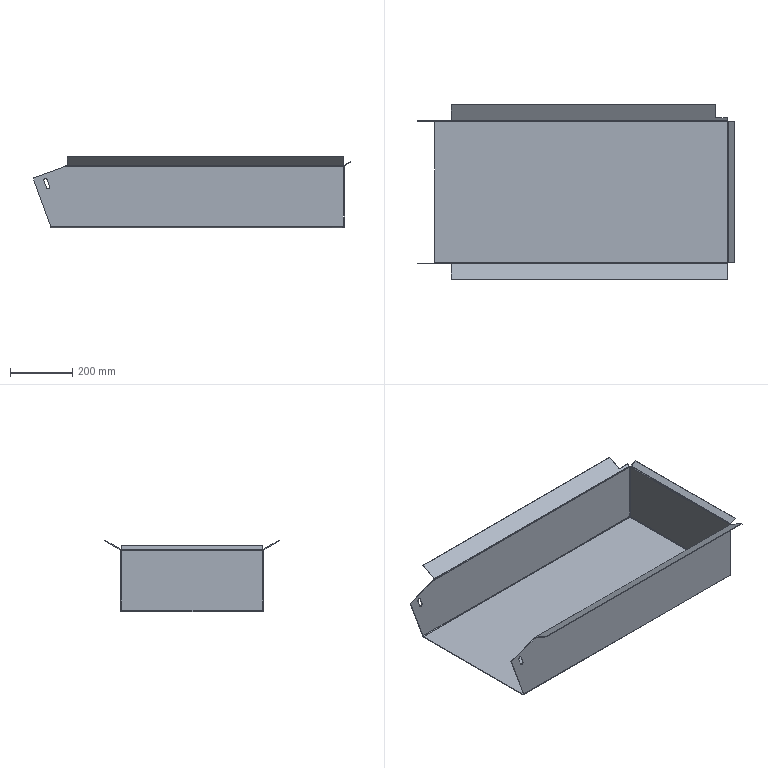Part | SolidWorks | features BaseBody 1 | 1 solid | 64 faces | box 1021 x 561.923 x 230 mm | volume 2027155 mm3 | plane 34 | cylinder 24 | spline 6 | commonest cylinder face diameters 8 x12 4 x6 11 x6